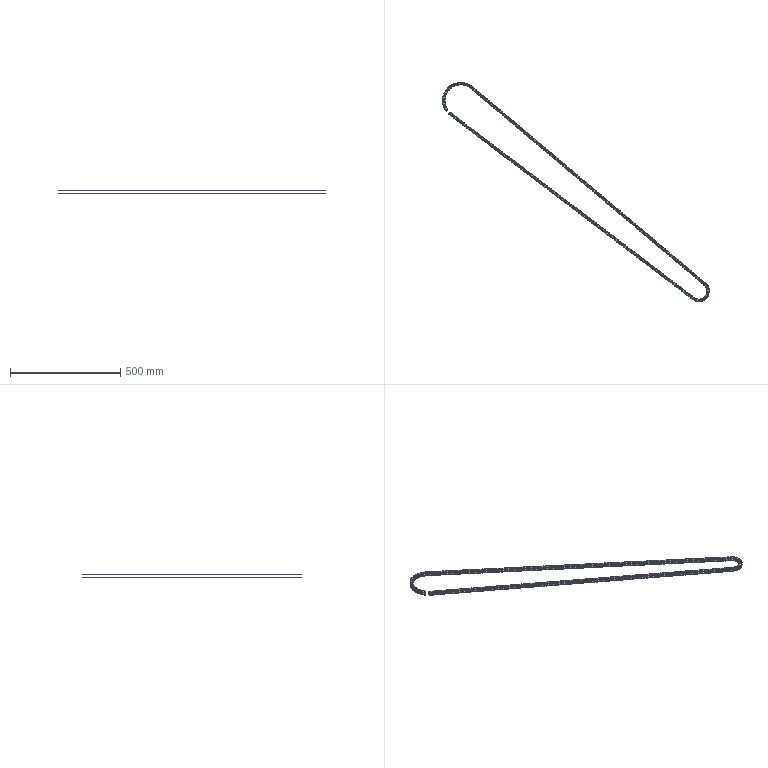Part | SolidWorks | features ReferencePattern 244, LocalChainPattern 1 | 246 solids | 2706 faces | box 1209 x 993.396 x 13.92 mm | volume 70663 mm3 | cylinder 2214 | plane 492 | commonest cylinder face diameters 4.45 x984 11.81 x738 57.066 x492